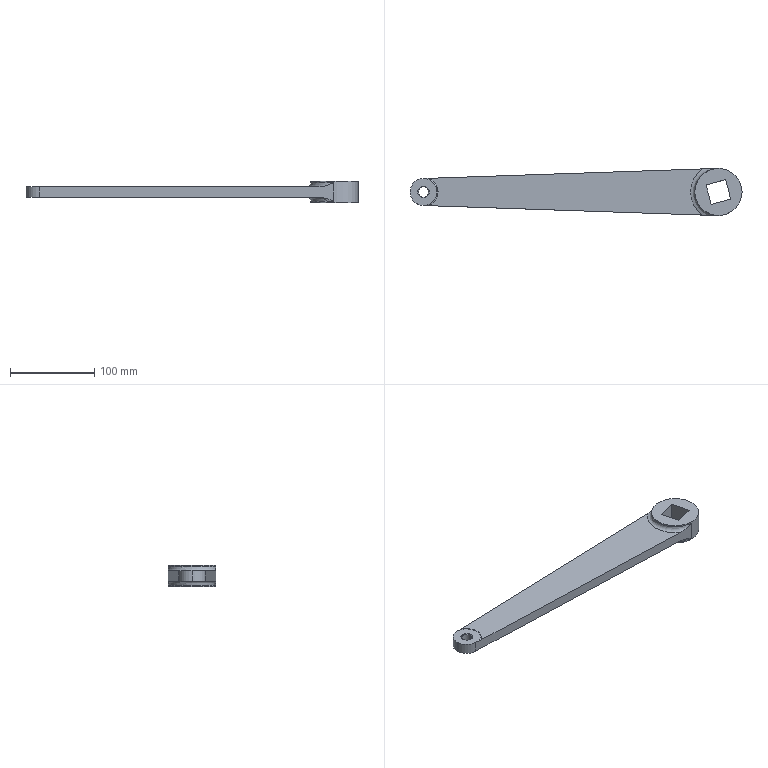Part | SolidWorks | features Boss 2, Fillet 2, Chamfer 1, Cut 1, Extrusion 1 | 1 solid | 28 faces | box 394 x 56 x 25 mm | volume 222247 mm3 | plane 12 | torus 6 | cylinder 6 | cone 4 | commonest cylinder face diameters 12 x2 32 x2 56 x2
STEP:
#1=CARTESIAN_POINT('',(-356.,0.,5.5));
#2=VERTEX_POINT('',#1);
#3=CARTESIAN_POINT('',(-344.,0.,5.5));
#4=VERTEX_POINT('',#3);
#5=CARTESIAN_POINT('',(-350.,0.,5.5));
#6=DIRECTION('',(0.,0.,1.));
#7=DIRECTION('',(1.,0.,0.));
#8=AXIS2_PLACEMENT_3D('',#5,#6,#7);
#9=CIRCLE('',#8,6.);
#10=EDGE_CURVE('',#2,#4,#9,.T.);
#11=ORIENTED_EDGE('',*,*,#10,.F.);
#12=CARTESIAN_POINT('',(-357.,0.,6.5));
#13=VERTEX_POINT('',#12);
#14=CARTESIAN_POINT('',(-356.,0.,5.5));
#15=DIRECTION('',(-0.7071,0.,0.7071));
#16=VECTOR('',#15,1000.);
#17=LINE('',#14,#16);
#18=EDGE_CURVE('',#2,#13,#17,.T.);
#19=ORIENTED_EDGE('',*,*,#18,.T.);
#20=CARTESIAN_POINT('',(-343.,0.,6.5));
#21=VERTEX_POINT('',#20);
#22=CARTESIAN_POINT('',(-350.,0.,6.5));
#23=DIRECTION('',(0.,0.,-1.));
#24=DIRECTION('',(1.,0.,0.));
#25=AXIS2_PLACEMENT_3D('',#22,#23,#24);
#26=CIRCLE('',#25,7.);
#27=EDGE_CURVE('',#21,#13,#26,.T.);
#28=ORIENTED_EDGE('',*,*,#27,.F.);
#29=CARTESIAN_POINT('',(-344.,0.,5.5));
#30=DIRECTION('',(0.7071,0.,0.7071));
#31=VECTOR('',#30,1000.);
#32=LINE('',#29,#31);
#33=EDGE_CURVE('',#4,#21,#32,.T.);
#34=ORIENTED_EDGE('',*,*,#33,.F.);
#35=EDGE_LOOP('',(#11,#19,#28,#34));
#36=FACE_OUTER_BOUND('',#35,.T.);
#37=CARTESIAN_POINT('',(-350.,0.,5.5));
#38=DIRECTION('',(0.,0.,1.));
#39=DIRECTION('',(1.,0.,0.));
#40=AXIS2_PLACEMENT_3D('',#37,#38,#39);
#41=CONICAL_SURFACE('',#40,6.,0.7854);
#42=ADVANCED_FACE('',(#36),#41,.F.);
#43=CARTESIAN_POINT('',(-344.,0.,-5.5));
#44=VERTEX_POINT('',#43);
#45=CARTESIAN_POINT('',(-356.,0.,-5.5));
#46=VERTEX_POINT('',#45);
#47=CARTESIAN_POINT('',(-350.,0.,-5.5));
#48=DIRECTION('',(0.,0.,-1.));
#49=DIRECTION('',(1.,0.,0.));
#50=AXIS2_PLACEMENT_3D('',#47,#48,#49);
#51=CIRCLE('',#50,6.);
#52=EDGE_CURVE('',#44,#46,#51,.T.);
#53=ORIENTED_EDGE('',*,*,#52,.F.);
#54=CARTESIAN_POINT('',(-343.,0.,-6.5));
#55=VERTEX_POINT('',#54);
#56=CARTESIAN_POINT('',(-343.,0.,-6.5));
#57=DIRECTION('',(0.7071,0.,-0.7071));
#58=VECTOR('',#57,1000.);
#59=LINE('',#56,#58);
#60=EDGE_CURVE('',#44,#55,#59,.T.);
#61=ORIENTED_EDGE('',*,*,#60,.T.);
#62=CARTESIAN_POINT('',(-357.,0.,-6.5));
#63=VERTEX_POINT('',#62);
#64=CARTESIAN_POINT('',(-350.,0.,-6.5));
#65=DIRECTION('',(0.,0.,1.));
#66=DIRECTION('',(1.,0.,0.));
#67=AXIS2_PLACEMENT_3D('',#64,#65,#66);
#68=CIRCLE('',#67,7.);
#69=EDGE_CURVE('',#63,#55,#68,.T.);
#70=ORIENTED_EDGE('',*,*,#69,.F.);
#71=CARTESIAN_POINT('',(-357.,0.,-6.5));
#72=DIRECTION('',(-0.7071,0.,-0.7071));
#73=VECTOR('',#72,1000.);
#74=LINE('',#71,#73);
#75=EDGE_CURVE('',#46,#63,#74,.T.);
#76=ORIENTED_EDGE('',*,*,#75,.F.);
#77=EDGE_LOOP('',(#53,#61,#70,#76));
#78=FACE_OUTER_BOUND('',#77,.T.);
#79=CARTESIAN_POINT('',(-350.,0.,-6.5));
#80=DIRECTION('',(0.,0.,-1.));
#81=DIRECTION('',(-1.,0.,0.));
#82=AXIS2_PLACEMENT_3D('',#79,#80,#81);
#83=CONICAL_SURFACE('',#82,7.,0.7854);
#84=ADVANCED_FACE('',(#78),#83,.F.);
#85=CARTESIAN_POINT('',(-332.677,0.,-6.));
#86=VERTEX_POINT('',#85);
#87=CARTESIAN_POINT('',(-343.913,16.218,-6.));
#88=VERTEX_POINT('',#87);
#89=CARTESIAN_POINT('',(-350.,0.,-6.));
#90=DIRECTION('',(0.,0.,1.));
#91=DIRECTION('',(1.,0.,0.));
#92=AXIS2_PLACEMENT_3D('',#89,#90,#91);
#93=CIRCLE('',#92,17.323);
#94=EDGE_CURVE('',#86,#88,#93,.T.);
#95=ORIENTED_EDGE('',*,*,#94,.F.);
#96=CARTESIAN_POINT('',(-334.,0.,-6.5));
#97=VERTEX_POINT('',#96);
#98=CARTESIAN_POINT('',(-332.677,0.,-8.));
#99=DIRECTION('',(0.,-1.,0.));
#100=DIRECTION('',(0.,0.,-1.));
#101=AXIS2_PLACEMENT_3D('',#98,#99,#100);
#102=CIRCLE('',#101,2.);
#103=EDGE_CURVE('',#86,#97,#102,.T.);
#104=ORIENTED_EDGE('',*,*,#103,.T.);
#105=CARTESIAN_POINT('',(-350.549,15.991,-6.5));
#106=VERTEX_POINT('',#105);
#107=CARTESIAN_POINT('',(-350.,0.,-6.5));
#108=DIRECTION('',(0.,0.,1.));
#109=DIRECTION('',(1.,0.,0.));
#110=AXIS2_PLACEMENT_3D('',#107,#108,#109);
#111=CIRCLE('',#110,16.);
#112=EDGE_CURVE('',#97,#106,#111,.T.);
#113=ORIENTED_EDGE('',*,*,#112,.T.);
#114=CARTESIAN_POINT('',(-343.913,16.218,-6.));
#115=CARTESIAN_POINT('',(-345.026,16.18,-6.));
#116=CARTESIAN_POINT('',(-346.129,16.142,-6.131));
#117=CARTESIAN_POINT('',(-347.783,16.085,-6.321));
#118=CARTESIAN_POINT('',(-348.334,16.067,-6.383));
#119=CARTESIAN_POINT('',(-349.439,16.029,-6.473));
#120=CARTESIAN_POINT('',(-349.993,16.01,-6.5));
#121=CARTESIAN_POINT('',(-350.549,15.991,-6.5));
#122=B_SPLINE_CURVE_WITH_KNOTS('',3,(#114,#115,#116,#117,#118,#119,#120,#121),.UNSPECIFIED.,.F.,.F.,(4,2,2,4),(0.,0.00333,0.004995,0.00666),.UNSPECIFIED.);
#123=EDGE_CURVE('',#88,#106,#122,.T.);
#124=ORIENTED_EDGE('',*,*,#123,.F.);
#125=EDGE_LOOP('',(#95,#104,#113,#124));
#126=FACE_OUTER_BOUND('',#125,.T.);
#127=CARTESIAN_POINT('',(-350.,0.,-8.));
#128=DIRECTION('',(0.,0.,1.));
#129=DIRECTION('',(1.,0.,0.));
#130=AXIS2_PLACEMENT_3D('',#127,#128,#129);
#131=TOROIDAL_SURFACE('',#130,17.323,2.);
#132=ADVANCED_FACE('',(#126),#131,.F.);
#133=CARTESIAN_POINT('',(-334.,0.,6.5));
#134=VERTEX_POINT('',#133);
#135=CARTESIAN_POINT('',(-350.549,15.991,6.5));
#136=VERTEX_POINT('',#135);
#137=CARTESIAN_POINT('',(-350.,0.,6.5));
#138=DIRECTION('',(0.,0.,1.));
#139=DIRECTION('',(1.,0.,0.));
#140=AXIS2_PLACEMENT_3D('',#137,#138,#139);
#141=CIRCLE('',#140,16.);
#142=EDGE_CURVE('',#134,#136,#141,.T.);
#143=ORIENTED_EDGE('',*,*,#142,.F.);
#144=CARTESIAN_POINT('',(-332.677,0.,6.));
#145=VERTEX_POINT('',#144);
#146=CARTESIAN_POINT('',(-332.677,0.,8.));
#147=DIRECTION('',(0.,-1.,0.));
#148=DIRECTION('',(0.,0.,-1.));
#149=AXIS2_PLACEMENT_3D('',#146,#147,#148);
#150=CIRCLE('',#149,2.);
#151=EDGE_CURVE('',#134,#145,#150,.T.);
#152=ORIENTED_EDGE('',*,*,#151,.T.);
#153=CARTESIAN_POINT('',(-343.913,16.218,6.));
#154=VERTEX_POINT('',#153);
#155=CARTESIAN_POINT('',(-350.,0.,6.));
#156=DIRECTION('',(0.,0.,-1.));
#157=DIRECTION('',(1.,0.,0.));
#158=AXIS2_PLACEMENT_3D('',#155,#156,#157);
#159=CIRCLE('',#158,17.323);
#160=EDGE_CURVE('',#154,#145,#159,.T.);
#161=ORIENTED_EDGE('',*,*,#160,.F.);
#162=CARTESIAN_POINT('',(-350.549,15.991,6.5));
#163=CARTESIAN_POINT('',(-349.992,16.01,6.5));
#164=CARTESIAN_POINT('',(-349.438,16.029,6.473));
#165=CARTESIAN_POINT('',(-348.332,16.067,6.383));
#166=CARTESIAN_POINT('',(-347.781,16.086,6.321));
#167=CARTESIAN_POINT('',(-346.127,16.142,6.131));
#168=CARTESIAN_POINT('',(-345.024,16.18,6.));
#169=CARTESIAN_POINT('',(-343.913,16.218,6.));
#170=B_SPLINE_CURVE_WITH_KNOTS('',3,(#162,#163,#164,#165,#166,#167,#168,#169),.UNSPECIFIED.,.F.,.F.,(4,2,2,4),(0.,0.001665,0.00333,0.006659),.UNSPECIFIED.);
#171=EDGE_CURVE('',#136,#154,#170,.T.);
#172=ORIENTED_EDGE('',*,*,#171,.F.);
#173=EDGE_LOOP('',(#143,#152,#161,#172));
#174=FACE_OUTER_BOUND('',#173,.T.);
#175=CARTESIAN_POINT('',(-350.,0.,8.));
#176=DIRECTION('',(0.,0.,1.));
#177=DIRECTION('',(1.,0.,0.));
#178=AXIS2_PLACEMENT_3D('',#175,#176,#177);
#179=TOROIDAL_SURFACE('',#178,17.323,2.);
#180=ADVANCED_FACE('',(#174),#179,.F.);
#181=ORIENTED_EDGE('',*,*,#52,.T.);
#182=CARTESIAN_POINT('',(-356.,0.,-12.5));
#183=DIRECTION('',(0.,0.,1.));
#184=VECTOR('',#183,1000.);
#185=LINE('',#182,#184);
#186=EDGE_CURVE('',#46,#2,#185,.T.);
#187=ORIENTED_EDGE('',*,*,#186,.T.);
#188=ORIENTED_EDGE('',*,*,#10,.T.);
#189=CARTESIAN_POINT('',(-344.,0.,-12.5));
#190=DIRECTION('',(0.,0.,1.));
#191=VECTOR('',#190,1000.);
#192=LINE('',#189,#191);
#193=EDGE_CURVE('',#44,#4,#192,.T.);
#194=ORIENTED_EDGE('',*,*,#193,.F.);
#195=EDGE_LOOP('',(#181,#187,#188,#194));
#196=FACE_OUTER_BOUND('',#195,.T.);
#197=CARTESIAN_POINT('',(-350.,0.,-12.5));
#198=DIRECTION('',(0.,0.,1.));
#199=DIRECTION('',(1.,0.,0.));
#200=AXIS2_PLACEMENT_3D('',#197,#198,#199);
#201=CYLINDRICAL_SURFACE('',#200,6.);
#202=ADVANCED_FACE('',(#196),#201,.F.);
#203=CARTESIAN_POINT('',(-366.,0.,6.5));
#204=VERTEX_POINT('',#203);
#205=CARTESIAN_POINT('',(-350.549,-15.991,6.5));
#206=VERTEX_POINT('',#205);
#207=CARTESIAN_POINT('',(-350.,0.,6.5));
#208=DIRECTION('',(0.,0.,1.));
#209=DIRECTION('',(1.,0.,0.));
#210=AXIS2_PLACEMENT_3D('',#207,#208,#209);
#211=CIRCLE('',#210,16.);
#212=EDGE_CURVE('',#204,#206,#211,.T.);
#213=ORIENTED_EDGE('',*,*,#212,.F.);
#214=CARTESIAN_POINT('',(-366.,0.,-6.5));
#215=VERTEX_POINT('',#214);
#216=CARTESIAN_POINT('',(-366.,0.,6.5));
#217=DIRECTION('',(0.,0.,-1.));
#218=VECTOR('',#217,1000.);
#219=LINE('',#216,#218);
#220=EDGE_CURVE('',#204,#215,#219,.T.);
#221=ORIENTED_EDGE('',*,*,#220,.T.);
#222=CARTESIAN_POINT('',(-350.549,-15.991,-6.5));
#223=VERTEX_POINT('',#222);
#224=CARTESIAN_POINT('',(-350.,0.,-6.5));
#225=DIRECTION('',(0.,0.,1.));
#226=DIRECTION('',(1.,0.,0.));
#227=AXIS2_PLACEMENT_3D('',#224,#225,#226);
#228=CIRCLE('',#227,16.);
#229=EDGE_CURVE('',#215,#223,#228,.T.);
#230=ORIENTED_EDGE('',*,*,#229,.T.);
#231=CARTESIAN_POINT('',(-350.549,-15.991,6.));
#232=DIRECTION('',(0.,0.,-1.));
#233=VECTOR('',#232,1000.);
#234=LINE('',#231,#233);
#235=EDGE_CURVE('',#206,#223,#234,.T.);
#236=ORIENTED_EDGE('',*,*,#235,.F.);
#237=EDGE_LOOP('',(#213,#221,#230,#236));
#238=FACE_OUTER_BOUND('',#237,.T.);
#239=CARTESIAN_POINT('',(-350.,0.,6.5));
#240=DIRECTION('',(0.,0.,-1.));
#241=DIRECTION('',(-1.,0.,0.));
#242=AXIS2_PLACEMENT_3D('',#239,#240,#241);
#243=CYLINDRICAL_SURFACE('',#242,16.);
#244=ADVANCED_FACE('',(#238),#243,.T.);
#245=CARTESIAN_POINT('',(28.,0.,12.5));
#246=VERTEX_POINT('',#245);
#247=CARTESIAN_POINT('',(-28.,0.,12.5));
#248=VERTEX_POINT('',#247);
#249=CARTESIAN_POINT('',(0.,0.,12.5));
#250=DIRECTION('',(0.,0.,1.));
#251=DIRECTION('',(1.,0.,0.));
#252=AXIS2_PLACEMENT_3D('',#249,#250,#251);
#253=CIRCLE('',#252,28.);
#254=EDGE_CURVE('',#246,#248,#253,.T.);
#255=ORIENTED_EDGE('',*,*,#254,.F.);
#256=CARTESIAN_POINT('',(28.,0.,-12.5));
#257=VERTEX_POINT('',#256);
#258=CARTESIAN_POINT('',(28.,0.,12.5));
#259=DIRECTION('',(0.,0.,-1.));
#260=VECTOR('',#259,1000.);
#261=LINE('',#258,#260);
#262=EDGE_CURVE('',#246,#257,#261,.T.);
#263=ORIENTED_EDGE('',*,*,#262,.T.);
#264=CARTESIAN_POINT('',(-28.,0.,-12.5));
#265=VERTEX_POINT('',#264);
#266=CARTESIAN_POINT('',(0.,0.,-12.5));
#267=DIRECTION('',(0.,0.,1.));
#268=DIRECTION('',(1.,0.,0.));
#269=AXIS2_PLACEMENT_3D('',#266,#267,#268);
#270=CIRCLE('',#269,28.);
#271=EDGE_CURVE('',#257,#265,#270,.T.);
#272=ORIENTED_EDGE('',*,*,#271,.T.);
#273=CARTESIAN_POINT('',(-28.,0.,-11.));
#274=VERTEX_POINT('',#273);
#275=CARTESIAN_POINT('',(-28.,0.,12.5));
#276=DIRECTION('',(0.,0.,-1.));
#277=VECTOR('',#276,1000.);
#278=LINE('',#275,#277);
#279=EDGE_CURVE('',#274,#265,#278,.T.);
#280=ORIENTED_EDGE('',*,*,#279,.F.);
#281=CARTESIAN_POINT('',(-0.96,27.984,-11.));
#282=VERTEX_POINT('',#281);
#283=CARTESIAN_POINT('',(0.,0.,-11.));
#284=DIRECTION('',(0.,0.,-1.));
#285=DIRECTION('',(1.,0.,0.));
#286=AXIS2_PLACEMENT_3D('',#283,#284,#285);
#287=CIRCLE('',#286,28.);
#288=EDGE_CURVE('',#274,#282,#287,.T.);
#289=ORIENTED_EDGE('',*,*,#288,.T.);
#290=CARTESIAN_POINT('',(-0.96,27.984,11.));
#291=VERTEX_POINT('',#290);
#292=CARTESIAN_POINT('',(-0.96,27.984,6.));
#293=DIRECTION('',(0.,0.,-1.));
#294=VECTOR('',#293,1000.);
#295=LINE('',#292,#294);
#296=EDGE_CURVE('',#291,#282,#295,.T.);
#297=ORIENTED_EDGE('',*,*,#296,.F.);
#298=CARTESIAN_POINT('',(-28.,0.,11.));
#299=VERTEX_POINT('',#298);
#300=CARTESIAN_POINT('',(0.,0.,11.));
#301=DIRECTION('',(0.,0.,1.));
#302=DIRECTION('',(1.,0.,0.));
#303=AXIS2_PLACEMENT_3D('',#300,#301,#302);
#304=CIRCLE('',#303,28.);
#305=EDGE_CURVE('',#291,#299,#304,.T.);
#306=ORIENTED_EDGE('',*,*,#305,.T.);
#307=CARTESIAN_POINT('',(-28.,0.,12.5));
#308=DIRECTION('',(0.,0.,-1.));
#309=VECTOR('',#308,1000.);
#310=LINE('',#307,#309);
#311=EDGE_CURVE('',#248,#299,#310,.T.);
#312=ORIENTED_EDGE('',*,*,#311,.F.);
#313=EDGE_LOOP('',(#255,#263,#272,#280,#289,#297,#306,#312));
#314=FACE_OUTER_BOUND('',#313,.T.);
#315=CARTESIAN_POINT('',(0.,0.,12.5));
#316=DIRECTION('',(0.,0.,-1.));
#317=DIRECTION('',(-1.,0.,0.));
#318=AXIS2_PLACEMENT_3D('',#315,#316,#317);
#319=CYLINDRICAL_SURFACE('',#318,28.);
#320=ADVANCED_FACE('',(#314),#319,.T.);
#321=CARTESIAN_POINT('',(-18.414,-27.385,-6.));
#322=VERTEX_POINT('',#321);
#323=CARTESIAN_POINT('',(-343.913,-16.218,-6.));
#324=VERTEX_POINT('',#323);
#325=CARTESIAN_POINT('',(-159.15,-22.557,-6.));
#326=DIRECTION('',(-0.9994,0.03429,0.));
#327=VECTOR('',#326,1000.);
#328=LINE('',#325,#327);
#329=EDGE_CURVE('',#322,#324,#328,.T.);
#330=ORIENTED_EDGE('',*,*,#329,.F.);
#331=CARTESIAN_POINT('',(-0.96,-27.984,-11.));
#332=VERTEX_POINT('',#331);
#333=CARTESIAN_POINT('',(-18.414,-27.385,-6.));
#334=CARTESIAN_POINT('',(-17.645,-27.411,-6.));
#335=CARTESIAN_POINT('',(-16.885,-27.437,-6.049));
#336=CARTESIAN_POINT('',(-15.376,-27.489,-6.219));
#337=CARTESIAN_POINT('',(-14.628,-27.515,-6.34));
#338=CARTESIAN_POINT('',(-13.141,-27.566,-6.639));
#339=CARTESIAN_POINT('',(-12.402,-27.591,-6.816));
#340=CARTESIAN_POINT('',(-10.932,-27.641,-7.215));
#341=CARTESIAN_POINT('',(-10.2,-27.667,-7.436));
#342=CARTESIAN_POINT('',(-8.025,-27.741,-8.147));
#343=CARTESIAN_POINT('',(-6.599,-27.79,-8.683));
#344=CARTESIAN_POINT('',(-4.476,-27.863,-9.53));
#345=CARTESIAN_POINT('',(-3.771,-27.887,-9.82));
#346=CARTESIAN_POINT('',(-2.716,-27.923,-10.26));
#347=CARTESIAN_POINT('',(-2.364,-27.935,-10.407));
#348=CARTESIAN_POINT('',(-1.662,-27.959,-10.703));
#349=CARTESIAN_POINT('',(-1.309,-27.972,-10.852));
#350=CARTESIAN_POINT('',(-0.96,-27.984,-11.));
#351=B_SPLINE_CURVE_WITH_KNOTS('',3,(#333,#334,#335,#336,#337,#338,#339,#340,#341,#342,#343,#344,#345,#346,#347,#348,#349,#350),.UNSPECIFIED.,.F.,.F.,(4,2,2,2,2,2,2,2,4),(0.,0.002275,0.00455,0.006826,0.009101,0.01365,0.01593,0.01706,0.0182),.UNSPECIFIED.);
#352=EDGE_CURVE('',#322,#332,#351,.T.);
#353=ORIENTED_EDGE('',*,*,#352,.T.);
#354=CARTESIAN_POINT('',(-0.96,-27.984,11.));
#355=VERTEX_POINT('',#354);
#356=CARTESIAN_POINT('',(-0.96,-27.984,6.));
#357=DIRECTION('',(0.,0.,-1.));
#358=VECTOR('',#357,1000.);
#359=LINE('',#356,#358);
#360=EDGE_CURVE('',#355,#332,#359,.T.);
#361=ORIENTED_EDGE('',*,*,#360,.F.);
#362=CARTESIAN_POINT('',(-18.414,-27.385,6.));
#363=VERTEX_POINT('',#362);
#364=CARTESIAN_POINT('',(-0.96,-27.984,11.));
#365=CARTESIAN_POINT('',(-2.363,-27.935,10.407));
#366=CARTESIAN_POINT('',(-3.768,-27.887,9.812));
#367=CARTESIAN_POINT('',(-6.599,-27.79,8.683));
#368=CARTESIAN_POINT('',(-8.025,-27.741,8.147));
#369=CARTESIAN_POINT('',(-10.2,-27.667,7.436));
#370=CARTESIAN_POINT('',(-10.932,-27.641,7.215));
#371=CARTESIAN_POINT('',(-12.402,-27.591,6.816));
#372=CARTESIAN_POINT('',(-13.141,-27.566,6.639));
#373=CARTESIAN_POINT('',(-14.628,-27.515,6.34));
#374=CARTESIAN_POINT('',(-15.376,-27.489,6.219));
#375=CARTESIAN_POINT('',(-16.885,-27.437,6.049));
#376=CARTESIAN_POINT('',(-17.645,-27.411,6.));
#377=CARTESIAN_POINT('',(-18.414,-27.385,6.));
#378=B_SPLINE_CURVE_WITH_KNOTS('',3,(#364,#365,#366,#367,#368,#369,#370,#371,#372,#373,#374,#375,#376,#377),.UNSPECIFIED.,.F.,.F.,(4,2,2,2,2,2,4),(-0.00003347,0.00454,0.009113,0.0114,0.01369,0.01597,0.01826),.UNSPECIFIED.);
#379=EDGE_CURVE('',#355,#363,#378,.T.);
#380=ORIENTED_EDGE('',*,*,#379,.T.);
#381=CARTESIAN_POINT('',(-343.913,-16.218,6.));
#382=VERTEX_POINT('',#381);
#383=CARTESIAN_POINT('',(-159.15,-22.557,6.));
#384=DIRECTION('',(-0.9994,0.03429,0.));
#385=VECTOR('',#384,1000.);
#386=LINE('',#383,#385);
#387=EDGE_CURVE('',#363,#382,#386,.T.);
#388=ORIENTED_EDGE('',*,*,#387,.T.);
#389=CARTESIAN_POINT('',(-343.913,-16.218,6.));
#390=CARTESIAN_POINT('',(-345.026,-16.18,6.));
#391=CARTESIAN_POINT('',(-346.129,-16.142,6.131));
#392=CARTESIAN_POINT('',(-347.783,-16.085,6.321));
#393=CARTESIAN_POINT('',(-348.334,-16.067,6.383));
#394=CARTESIAN_POINT('',(-349.439,-16.029,6.473));
#395=CARTESIAN_POINT('',(-349.993,-16.01,6.5));
#396=CARTESIAN_POINT('',(-350.549,-15.991,6.5));
#397=B_SPLINE_CURVE_WITH_KNOTS('',3,(#389,#390,#391,#392,#393,#394,#395,#396),.UNSPECIFIED.,.F.,.F.,(4,2,2,4),(0.,0.00333,0.004995,0.00666),.UNSPECIFIED.);
#398=EDGE_CURVE('',#382,#206,#397,.T.);
#399=ORIENTED_EDGE('',*,*,#398,.T.);
#400=ORIENTED_EDGE('',*,*,#235,.T.);
#401=CARTESIAN_POINT('',(-350.549,-15.991,-6.5));
#402=CARTESIAN_POINT('',(-349.992,-16.01,-6.5));
#403=CARTESIAN_POINT('',(-349.438,-16.029,-6.473));
#404=CARTESIAN_POINT('',(-348.332,-16.067,-6.383));
#405=CARTESIAN_POINT('',(-347.781,-16.086,-6.321));
#406=CARTESIAN_POINT('',(-346.127,-16.142,-6.131));
#407=CARTESIAN_POINT('',(-345.024,-16.18,-6.));
#408=CARTESIAN_POINT('',(-343.913,-16.218,-6.));
#409=B_SPLINE_CURVE_WITH_KNOTS('',3,(#401,#402,#403,#404,#405,#406,#407,#408),.UNSPECIFIED.,.F.,.F.,(4,2,2,4),(0.,0.001665,0.00333,0.006659),.UNSPECIFIED.);
#410=EDGE_CURVE('',#223,#324,#409,.T.);
#411=ORIENTED_EDGE('',*,*,#410,.T.);
#412=EDGE_LOOP('',(#330,#353,#361,#380,#388,#399,#400,#411));
#413=FACE_OUTER_BOUND('',#412,.T.);
#414=CARTESIAN_POINT('',(-159.15,-22.557,6.));
#415=DIRECTION('',(-0.03429,-0.9994,0.));
#416=DIRECTION('',(0.9994,-0.03429,0.));
#417=AXIS2_PLACEMENT_3D('',#414,#415,#416);
#418=PLANE('',#417);
#419=ADVANCED_FACE('',(#413),#418,.T.);
#420=ORIENTED_EDGE('',*,*,#296,.T.);
#421=CARTESIAN_POINT('',(-18.414,27.385,-6.));
#422=VERTEX_POINT('',#421);
#423=CARTESIAN_POINT('',(-0.96,27.984,-11.));
#424=CARTESIAN_POINT('',(-2.363,27.935,-10.407));
#425=CARTESIAN_POINT('',(-3.768,27.887,-9.812));
#426=CARTESIAN_POINT('',(-6.599,27.79,-8.683));
#427=CARTESIAN_POINT('',(-8.025,27.741,-8.147));
#428=CARTESIAN_POINT('',(-10.2,27.667,-7.436));
#429=CARTESIAN_POINT('',(-10.932,27.641,-7.215));
#430=CARTESIAN_POINT('',(-12.402,27.591,-6.816));
#431=CARTESIAN_POINT('',(-13.141,27.566,-6.639));
#432=CARTESIAN_POINT('',(-14.628,27.515,-6.34));
#433=CARTESIAN_POINT('',(-15.376,27.489,-6.219));
#434=CARTESIAN_POINT('',(-16.885,27.437,-6.049));
#435=CARTESIAN_POINT('',(-17.645,27.411,-6.));
#436=CARTESIAN_POINT('',(-18.414,27.385,-6.));
#437=B_SPLINE_CURVE_WITH_KNOTS('',3,(#423,#424,#425,#426,#427,#428,#429,#430,#431,#432,#433,#434,#435,#436),.UNSPECIFIED.,.F.,.F.,(4,2,2,2,2,2,4),(-0.00003347,0.00454,0.009113,0.0114,0.01369,0.01597,0.01826),.UNSPECIFIED.);
#438=EDGE_CURVE('',#282,#422,#437,.T.);
#439=ORIENTED_EDGE('',*,*,#438,.T.);
#440=CARTESIAN_POINT('',(-180.373,21.829,-6.));
#441=DIRECTION('',(-0.9994,-0.03429,0.));
#442=VECTOR('',#441,1000.);
#443=LINE('',#440,#442);
#444=EDGE_CURVE('',#422,#88,#443,.T.);
#445=ORIENTED_EDGE('',*,*,#444,.T.);
#446=ORIENTED_EDGE('',*,*,#123,.T.);
#447=CARTESIAN_POINT('',(-350.549,15.991,6.));
#448=DIRECTION('',(0.,0.,-1.));
#449=VECTOR('',#448,1000.);
#450=LINE('',#447,#449);
#451=EDGE_CURVE('',#136,#106,#450,.T.);
#452=ORIENTED_EDGE('',*,*,#451,.F.);
#453=ORIENTED_EDGE('',*,*,#171,.T.);
#454=CARTESIAN_POINT('',(-18.414,27.385,6.));
#455=VERTEX_POINT('',#454);
#456=CARTESIAN_POINT('',(-180.373,21.829,6.));
#457=DIRECTION('',(-0.9994,-0.03429,0.));
#458=VECTOR('',#457,1000.);
#459=LINE('',#456,#458);
#460=EDGE_CURVE('',#455,#154,#459,.T.);
#461=ORIENTED_EDGE('',*,*,#460,.F.);
#462=CARTESIAN_POINT('',(-18.414,27.385,6.));
#463=CARTESIAN_POINT('',(-17.645,27.411,6.));
#464=CARTESIAN_POINT('',(-16.885,27.437,6.049));
#465=CARTESIAN_POINT('',(-15.376,27.489,6.219));
#466=CARTESIAN_POINT('',(-14.628,27.515,6.34));
#467=CARTESIAN_POINT('',(-13.141,27.566,6.639));
#468=CARTESIAN_POINT('',(-12.402,27.591,6.816));
#469=CARTESIAN_POINT('',(-10.932,27.641,7.215));
#470=CARTESIAN_POINT('',(-10.2,27.667,7.436));
#471=CARTESIAN_POINT('',(-8.025,27.741,8.147));
#472=CARTESIAN_POINT('',(-6.599,27.79,8.683));
#473=CARTESIAN_POINT('',(-4.476,27.863,9.53));
#474=CARTESIAN_POINT('',(-3.771,27.887,9.82));
#475=CARTESIAN_POINT('',(-2.716,27.923,10.26));
#476=CARTESIAN_POINT('',(-2.364,27.935,10.407));
#477=CARTESIAN_POINT('',(-1.662,27.959,10.703));
#478=CARTESIAN_POINT('',(-1.309,27.972,10.852));
#479=CARTESIAN_POINT('',(-0.96,27.984,11.));
#480=B_SPLINE_CURVE_WITH_KNOTS('',3,(#462,#463,#464,#465,#466,#467,#468,#469,#470,#471,#472,#473,#474,#475,#476,#477,#478,#479),.UNSPECIFIED.,.F.,.F.,(4,2,2,2,2,2,2,2,4),(0.,0.002275,0.00455,0.006826,0.009101,0.01365,0.01593,0.01706,0.0182),.UNSPECIFIED.);
#481=EDGE_CURVE('',#455,#291,#480,.T.);
#482=ORIENTED_EDGE('',*,*,#481,.T.);
#483=EDGE_LOOP('',(#420,#439,#445,#446,#452,#453,#461,#482));
#484=FACE_OUTER_BOUND('',#483,.T.);
#485=CARTESIAN_POINT('',(-180.373,21.829,6.));
#486=DIRECTION('',(0.03429,-0.9994,0.));
#487=DIRECTION('',(0.9994,0.03429,0.));
#488=AXIS2_PLACEMENT_3D('',#485,#486,#487);
#489=PLANE('',#488);
#490=ADVANCED_FACE('',(#484),#489,.F.);
#491=ORIENTED_EDGE('',*,*,#460,.T.);
#492=ORIENTED_EDGE('',*,*,#160,.T.);
#493=CARTESIAN_POINT('',(-350.,0.,6.));
#494=DIRECTION('',(0.,0.,-1.));
#495=DIRECTION('',(1.,0.,0.));
#496=AXIS2_PLACEMENT_3D('',#493,#494,#495);
#497=CIRCLE('',#496,17.323);
#498=EDGE_CURVE('',#145,#382,#497,.T.);
#499=ORIENTED_EDGE('',*,*,#498,.T.);
#500=ORIENTED_EDGE('',*,*,#387,.F.);
#501=CARTESIAN_POINT('',(0.,0.,6.));
#502=DIRECTION('',(0.,0.,-1.));
#503=DIRECTION('',(1.,0.,0.));
#504=AXIS2_PLACEMENT_3D('',#501,#502,#503);
#505=CIRCLE('',#504,33.);
#506=EDGE_CURVE('',#363,#455,#505,.T.);
#507=ORIENTED_EDGE('',*,*,#506,.T.);
#508=EDGE_LOOP('',(#491,#492,#499,#500,#507));
#509=FACE_OUTER_BOUND('',#508,.T.);
#510=CARTESIAN_POINT('',(-169.,-309.681,6.));
#511=DIRECTION('',(0.,0.,1.));
#512=DIRECTION('',(1.,0.,0.));
#513=AXIS2_PLACEMENT_3D('',#510,#511,#512);
#514=PLANE('',#513);
#515=ADVANCED_FACE('',(#509),#514,.T.);
#516=ORIENTED_EDGE('',*,*,#329,.T.);
#517=CARTESIAN_POINT('',(-350.,0.,-6.));
#518=DIRECTION('',(0.,0.,1.));
#519=DIRECTION('',(1.,0.,0.));
#520=AXIS2_PLACEMENT_3D('',#517,#518,#519);
#521=CIRCLE('',#520,17.323);
#522=EDGE_CURVE('',#324,#86,#521,.T.);
#523=ORIENTED_EDGE('',*,*,#522,.T.);
#524=ORIENTED_EDGE('',*,*,#94,.T.);
#525=ORIENTED_EDGE('',*,*,#444,.F.);
#526=CARTESIAN_POINT('',(0.,0.,-6.));
#527=DIRECTION('',(0.,0.,1.));
#528=DIRECTION('',(1.,0.,0.));
#529=AXIS2_PLACEMENT_3D('',#526,#527,#528);
#530=CIRCLE('',#529,33.);
#531=EDGE_CURVE('',#422,#322,#530,.T.);
#532=ORIENTED_EDGE('',*,*,#531,.T.);
#533=EDGE_LOOP('',(#516,#523,#524,#525,#532));
#534=FACE_OUTER_BOUND('',#533,.T.);
#535=CARTESIAN_POINT('',(-169.,-309.681,-6.));
#536=DIRECTION('',(0.,0.,1.));
#537=DIRECTION('',(1.,0.,0.));
#538=AXIS2_PLACEMENT_3D('',#535,#536,#537);
#539=PLANE('',#538);
#540=ADVANCED_FACE('',(#534),#539,.F.);
#541=ORIENTED_EDGE('',*,*,#262,.F.);
#542=CARTESIAN_POINT('',(0.,0.,12.5));
#543=DIRECTION('',(0.,0.,1.));
#544=DIRECTION('',(1.,0.,0.));
#545=AXIS2_PLACEMENT_3D('',#542,#543,#544);
#546=CIRCLE('',#545,28.);
#547=EDGE_CURVE('',#248,#246,#546,.T.);
#548=ORIENTED_EDGE('',*,*,#547,.F.);
#549=ORIENTED_EDGE('',*,*,#311,.T.);
#550=CARTESIAN_POINT('',(0.,0.,11.));
#551=DIRECTION('',(0.,0.,1.));
#552=DIRECTION('',(1.,0.,0.));
#553=AXIS2_PLACEMENT_3D('',#550,#551,#552);
#554=CIRCLE('',#553,28.);
#555=EDGE_CURVE('',#299,#355,#554,.T.);
#556=ORIENTED_EDGE('',*,*,#555,.T.);
#557=ORIENTED_EDGE('',*,*,#360,.T.);
#558=CARTESIAN_POINT('',(0.,0.,-11.));
#559=DIRECTION('',(0.,0.,-1.));
#560=DIRECTION('',(1.,0.,0.));
#561=AXIS2_PLACEMENT_3D('',#558,#559,#560);
#562=CIRCLE('',#561,28.);
#563=EDGE_CURVE('',#332,#274,#562,.T.);
#564=ORIENTED_EDGE('',*,*,#563,.T.);
#565=ORIENTED_EDGE('',*,*,#279,.T.);
#566=CARTESIAN_POINT('',(0.,0.,-12.5));
#567=DIRECTION('',(0.,0.,1.));
#568=DIRECTION('',(1.,0.,0.));
#569=AXIS2_PLACEMENT_3D('',#566,#567,#568);
#570=CIRCLE('',#569,28.);
#571=EDGE_CURVE('',#265,#257,#570,.T.);
#572=ORIENTED_EDGE('',*,*,#571,.T.);
#573=EDGE_LOOP('',(#541,#548,#549,#556,#557,#564,#565,#572));
#574=FACE_OUTER_BOUND('',#573,.T.);
#575=CARTESIAN_POINT('',(0.,0.,12.5));
#576=DIRECTION('',(0.,0.,-1.));
#577=DIRECTION('',(-1.,0.,0.));
#578=AXIS2_PLACEMENT_3D('',#575,#576,#577);
#579=CYLINDRICAL_SURFACE('',#578,28.);
#580=ADVANCED_FACE('',(#574),#579,.T.);
#581=CARTESIAN_POINT('',(-14.697,8.485,12.5));
#582=VERTEX_POINT('',#581);
#583=CARTESIAN_POINT('',(-8.485,-14.697,12.5));
#584=VERTEX_POINT('',#583);
#585=CARTESIAN_POINT('',(-14.697,8.485,12.5));
#586=DIRECTION('',(0.2588,-0.9659,0.));
#587=VECTOR('',#586,1000.);
#588=LINE('',#585,#587);
#589=EDGE_CURVE('',#582,#584,#588,.T.);
#590=ORIENTED_EDGE('',*,*,#589,.F.);
#591=CARTESIAN_POINT('',(8.485,14.697,12.5));
#592=VERTEX_POINT('',#591);
#593=CARTESIAN_POINT('',(-14.697,8.485,12.5));
#594=DIRECTION('',(-0.9659,-0.2588,0.));
#595=VECTOR('',#594,1000.);
#596=LINE('',#593,#595);
#597=EDGE_CURVE('',#592,#582,#596,.T.);
#598=ORIENTED_EDGE('',*,*,#597,.F.);
#599=CARTESIAN_POINT('',(14.697,-8.485,12.5));
#600=VERTEX_POINT('',#599);
#601=CARTESIAN_POINT('',(8.485,14.697,12.5));
#602=DIRECTION('',(-0.2588,0.9659,0.));
#603=VECTOR('',#602,1000.);
#604=LINE('',#601,#603);
#605=EDGE_CURVE('',#600,#592,#604,.T.);
#606=ORIENTED_EDGE('',*,*,#605,.F.);
#607=CARTESIAN_POINT('',(-8.485,-14.697,12.5));
#608=DIRECTION('',(0.9659,0.2588,0.));
#609=VECTOR('',#608,1000.);
#610=LINE('',#607,#609);
#611=EDGE_CURVE('',#584,#600,#610,.T.);
#612=ORIENTED_EDGE('',*,*,#611,.F.);
#613=EDGE_LOOP('',(#590,#598,#606,#612));
#614=FACE_BOUND('',#613,.T.);
#615=ORIENTED_EDGE('',*,*,#547,.T.);
#616=ORIENTED_EDGE('',*,*,#254,.T.);
#617=EDGE_LOOP('',(#615,#616));
#618=FACE_OUTER_BOUND('',#617,.T.);
#619=CARTESIAN_POINT('',(-169.,-309.681,12.5));
#620=DIRECTION('',(0.,0.,1.));
#621=DIRECTION('',(1.,0.,0.));
#622=AXIS2_PLACEMENT_3D('',#619,#620,#621);
#623=PLANE('',#622);
#624=ADVANCED_FACE('',(#614,#618),#623,.T.);
#625=CARTESIAN_POINT('',(8.485,14.697,-12.5));
#626=VERTEX_POINT('',#625);
#627=CARTESIAN_POINT('',(-14.697,8.485,-12.5));
#628=VERTEX_POINT('',#627);
#629=CARTESIAN_POINT('',(-14.697,8.485,-12.5));
#630=DIRECTION('',(-0.9659,-0.2588,0.));
#631=VECTOR('',#630,1000.);
#632=LINE('',#629,#631);
#633=EDGE_CURVE('',#626,#628,#632,.T.);
#634=ORIENTED_EDGE('',*,*,#633,.T.);
#635=CARTESIAN_POINT('',(-8.485,-14.697,-12.5));
#636=VERTEX_POINT('',#635);
#637=CARTESIAN_POINT('',(-14.697,8.485,-12.5));
#638=DIRECTION('',(0.2588,-0.9659,0.));
#639=VECTOR('',#638,1000.);
#640=LINE('',#637,#639);
#641=EDGE_CURVE('',#628,#636,#640,.T.);
#642=ORIENTED_EDGE('',*,*,#641,.T.);
#643=CARTESIAN_POINT('',(14.697,-8.485,-12.5));
#644=VERTEX_POINT('',#643);
#645=CARTESIAN_POINT('',(-8.485,-14.697,-12.5));
#646=DIRECTION('',(0.9659,0.2588,0.));
#647=VECTOR('',#646,1000.);
#648=LINE('',#645,#647);
#649=EDGE_CURVE('',#636,#644,#648,.T.);
#650=ORIENTED_EDGE('',*,*,#649,.T.);
#651=CARTESIAN_POINT('',(8.485,14.697,-12.5));
#652=DIRECTION('',(-0.2588,0.9659,0.));
#653=VECTOR('',#652,1000.);
#654=LINE('',#651,#653);
#655=EDGE_CURVE('',#644,#626,#654,.T.);
#656=ORIENTED_EDGE('',*,*,#655,.T.);
#657=EDGE_LOOP('',(#634,#642,#650,#656));
#658=FACE_BOUND('',#657,.T.);
#659=ORIENTED_EDGE('',*,*,#571,.F.);
#660=ORIENTED_EDGE('',*,*,#271,.F.);
#661=EDGE_LOOP('',(#659,#660));
#662=FACE_OUTER_BOUND('',#661,.T.);
#663=CARTESIAN_POINT('',(-169.,-309.681,-12.5));
#664=DIRECTION('',(0.,0.,1.));
#665=DIRECTION('',(1.,0.,0.));
#666=AXIS2_PLACEMENT_3D('',#663,#664,#665);
#667=PLANE('',#666);
#668=ADVANCED_FACE('',(#658,#662),#667,.F.);
#669=ORIENTED_EDGE('',*,*,#220,.F.);
#670=CARTESIAN_POINT('',(-350.,0.,6.5));
#671=DIRECTION('',(0.,0.,1.));
#672=DIRECTION('',(1.,0.,0.));
#673=AXIS2_PLACEMENT_3D('',#670,#671,#672);
#674=CIRCLE('',#673,16.);
#675=EDGE_CURVE('',#136,#204,#674,.T.);
#676=ORIENTED_EDGE('',*,*,#675,.F.);
#677=ORIENTED_EDGE('',*,*,#451,.T.);
#678=CARTESIAN_POINT('',(-350.,0.,-6.5));
#679=DIRECTION('',(0.,0.,1.));
#680=DIRECTION('',(1.,0.,0.));
#681=AXIS2_PLACEMENT_3D('',#678,#679,#680);
#682=CIRCLE('',#681,16.);
#683=EDGE_CURVE('',#106,#215,#682,.T.);
#684=ORIENTED_EDGE('',*,*,#683,.T.);
#685=EDGE_LOOP('',(#669,#676,#677,#684));
#686=FACE_OUTER_BOUND('',#685,.T.);
#687=CARTESIAN_POINT('',(-350.,0.,6.5));
#688=DIRECTION('',(0.,0.,-1.));
#689=DIRECTION('',(-1.,0.,0.));
#690=AXIS2_PLACEMENT_3D('',#687,#688,#689);
#691=CYLINDRICAL_SURFACE('',#690,16.);
#692=ADVANCED_FACE('',(#686),#691,.T.);
#693=ORIENTED_EDGE('',*,*,#27,.T.);
#694=CARTESIAN_POINT('',(-350.,0.,6.5));
#695=DIRECTION('',(0.,0.,-1.));
#696=DIRECTION('',(1.,0.,0.));
#697=AXIS2_PLACEMENT_3D('',#694,#695,#696);
#698=CIRCLE('',#697,7.);
#699=EDGE_CURVE('',#13,#21,#698,.T.);
#700=ORIENTED_EDGE('',*,*,#699,.T.);
#701=EDGE_LOOP('',(#693,#700));
#702=FACE_BOUND('',#701,.T.);
#703=ORIENTED_EDGE('',*,*,#675,.T.);
#704=ORIENTED_EDGE('',*,*,#212,.T.);
#705=CARTESIAN_POINT('',(-350.,0.,6.5));
#706=DIRECTION('',(0.,0.,1.));
#707=DIRECTION('',(1.,0.,0.));
#708=AXIS2_PLACEMENT_3D('',#705,#706,#707);
#709=CIRCLE('',#708,16.);
#710=EDGE_CURVE('',#206,#134,#709,.T.);
#711=ORIENTED_EDGE('',*,*,#710,.T.);
#712=ORIENTED_EDGE('',*,*,#142,.T.);
#713=EDGE_LOOP('',(#703,#704,#711,#712));
#714=FACE_OUTER_BOUND('',#713,.T.);
#715=CARTESIAN_POINT('',(-169.,-309.681,6.5));
#716=DIRECTION('',(0.,0.,1.));
#717=DIRECTION('',(1.,0.,0.));
#718=AXIS2_PLACEMENT_3D('',#715,#716,#717);
#719=PLANE('',#718);
#720=ADVANCED_FACE('',(#702,#714),#719,.T.);
#721=ORIENTED_EDGE('',*,*,#69,.T.);
#722=CARTESIAN_POINT('',(-350.,0.,-6.5));
#723=DIRECTION('',(0.,0.,1.));
#724=DIRECTION('',(1.,0.,0.));
#725=AXIS2_PLACEMENT_3D('',#722,#723,#724);
#726=CIRCLE('',#725,7.);
#727=EDGE_CURVE('',#55,#63,#726,.T.);
#728=ORIENTED_EDGE('',*,*,#727,.T.);
#729=EDGE_LOOP('',(#721,#728));
#730=FACE_BOUND('',#729,.T.);
#731=ORIENTED_EDGE('',*,*,#683,.F.);
#732=ORIENTED_EDGE('',*,*,#112,.F.);
#733=CARTESIAN_POINT('',(-350.,0.,-6.5));
#734=DIRECTION('',(0.,0.,1.));
#735=DIRECTION('',(1.,0.,0.));
#736=AXIS2_PLACEMENT_3D('',#733,#734,#735);
#737=CIRCLE('',#736,16.);
#738=EDGE_CURVE('',#223,#97,#737,.T.);
#739=ORIENTED_EDGE('',*,*,#738,.F.);
#740=ORIENTED_EDGE('',*,*,#229,.F.);
#741=EDGE_LOOP('',(#731,#732,#739,#740));
#742=FACE_OUTER_BOUND('',#741,.T.);
#743=CARTESIAN_POINT('',(-169.,-309.681,-6.5));
#744=DIRECTION('',(0.,0.,1.));
#745=DIRECTION('',(1.,0.,0.));
#746=AXIS2_PLACEMENT_3D('',#743,#744,#745);
#747=PLANE('',#746);
#748=ADVANCED_FACE('',(#730,#742),#747,.F.);
#749=ORIENTED_EDGE('',*,*,#589,.T.);
#750=CARTESIAN_POINT('',(-8.485,-14.697,-12.5));
#751=DIRECTION('',(0.,0.,1.));
#752=VECTOR('',#751,1000.);
#753=LINE('',#750,#752);
#754=EDGE_CURVE('',#636,#584,#753,.T.);
#755=ORIENTED_EDGE('',*,*,#754,.F.);
#756=ORIENTED_EDGE('',*,*,#641,.F.);
#757=CARTESIAN_POINT('',(-14.697,8.485,-12.5));
#758=DIRECTION('',(0.,0.,1.));
#759=VECTOR('',#758,1000.);
#760=LINE('',#757,#759);
#761=EDGE_CURVE('',#628,#582,#760,.T.);
#762=ORIENTED_EDGE('',*,*,#761,.T.);
#763=EDGE_LOOP('',(#749,#755,#756,#762));
#764=FACE_OUTER_BOUND('',#763,.T.);
#765=CARTESIAN_POINT('',(-14.697,8.485,-12.5));
#766=DIRECTION('',(-0.9659,-0.2588,0.));
#767=DIRECTION('',(0.2588,-0.9659,0.));
#768=AXIS2_PLACEMENT_3D('',#765,#766,#767);
#769=PLANE('',#768);
#770=ADVANCED_FACE('',(#764),#769,.F.);
#771=ORIENTED_EDGE('',*,*,#597,.T.);
#772=ORIENTED_EDGE('',*,*,#761,.F.);
#773=ORIENTED_EDGE('',*,*,#633,.F.);
#774=CARTESIAN_POINT('',(8.485,14.697,-12.5));
#775=DIRECTION('',(0.,0.,1.));
#776=VECTOR('',#775,1000.);
#777=LINE('',#774,#776);
#778=EDGE_CURVE('',#626,#592,#777,.T.);
#779=ORIENTED_EDGE('',*,*,#778,.T.);
#780=EDGE_LOOP('',(#771,#772,#773,#779));
#781=FACE_OUTER_BOUND('',#780,.T.);
#782=CARTESIAN_POINT('',(-14.697,8.485,-12.5));
#783=DIRECTION('',(-0.2588,0.9659,0.));
#784=DIRECTION('',(-0.9659,-0.2588,0.));
#785=AXIS2_PLACEMENT_3D('',#782,#783,#784);
#786=PLANE('',#785);
#787=ADVANCED_FACE('',(#781),#786,.F.);
#788=ORIENTED_EDGE('',*,*,#605,.T.);
#789=ORIENTED_EDGE('',*,*,#778,.F.);
#790=ORIENTED_EDGE('',*,*,#655,.F.);
#791=CARTESIAN_POINT('',(14.697,-8.485,-12.5));
#792=DIRECTION('',(0.,0.,1.));
#793=VECTOR('',#792,1000.);
#794=LINE('',#791,#793);
#795=EDGE_CURVE('',#644,#600,#794,.T.);
#796=ORIENTED_EDGE('',*,*,#795,.T.);
#797=EDGE_LOOP('',(#788,#789,#790,#796));
#798=FACE_OUTER_BOUND('',#797,.T.);
#799=CARTESIAN_POINT('',(8.485,14.697,-12.5));
#800=DIRECTION('',(0.9659,0.2588,0.));
#801=DIRECTION('',(-0.2588,0.9659,0.));
#802=AXIS2_PLACEMENT_3D('',#799,#800,#801);
#803=PLANE('',#802);
#804=ADVANCED_FACE('',(#798),#803,.F.);
#805=ORIENTED_EDGE('',*,*,#611,.T.);
#806=ORIENTED_EDGE('',*,*,#795,.F.);
#807=ORIENTED_EDGE('',*,*,#649,.F.);
#808=ORIENTED_EDGE('',*,*,#754,.T.);
#809=EDGE_LOOP('',(#805,#806,#807,#808));
#810=FACE_OUTER_BOUND('',#809,.T.);
#811=CARTESIAN_POINT('',(-8.485,-14.697,-12.5));
#812=DIRECTION('',(0.2588,-0.9659,0.));
#813=DIRECTION('',(0.9659,0.2588,0.));
#814=AXIS2_PLACEMENT_3D('',#811,#812,#813);
#815=PLANE('',#814);
#816=ADVANCED_FACE('',(#810),#815,.F.);
#817=ORIENTED_EDGE('',*,*,#186,.F.);
#818=CARTESIAN_POINT('',(-350.,0.,-5.5));
#819=DIRECTION('',(0.,0.,-1.));
#820=DIRECTION('',(1.,0.,0.));
#821=AXIS2_PLACEMENT_3D('',#818,#819,#820);
#822=CIRCLE('',#821,6.);
#823=EDGE_CURVE('',#46,#44,#822,.T.);
#824=ORIENTED_EDGE('',*,*,#823,.T.);
#825=ORIENTED_EDGE('',*,*,#193,.T.);
#826=CARTESIAN_POINT('',(-350.,0.,5.5));
#827=DIRECTION('',(0.,0.,1.));
#828=DIRECTION('',(1.,0.,0.));
#829=AXIS2_PLACEMENT_3D('',#826,#827,#828);
#830=CIRCLE('',#829,6.);
#831=EDGE_CURVE('',#4,#2,#830,.T.);
#832=ORIENTED_EDGE('',*,*,#831,.T.);
#833=EDGE_LOOP('',(#817,#824,#825,#832));
#834=FACE_OUTER_BOUND('',#833,.T.);
#835=CARTESIAN_POINT('',(-350.,0.,-12.5));
#836=DIRECTION('',(0.,0.,1.));
#837=DIRECTION('',(1.,0.,0.));
#838=AXIS2_PLACEMENT_3D('',#835,#836,#837);
#839=CYLINDRICAL_SURFACE('',#838,6.);
#840=ADVANCED_FACE('',(#834),#839,.F.);
#841=ORIENTED_EDGE('',*,*,#438,.F.);
#842=ORIENTED_EDGE('',*,*,#288,.F.);
#843=ORIENTED_EDGE('',*,*,#563,.F.);
#844=ORIENTED_EDGE('',*,*,#352,.F.);
#845=ORIENTED_EDGE('',*,*,#531,.F.);
#846=EDGE_LOOP('',(#841,#842,#843,#844,#845));
#847=FACE_OUTER_BOUND('',#846,.T.);
#848=CARTESIAN_POINT('',(0.,0.,-11.));
#849=DIRECTION('',(0.,0.,1.));
#850=DIRECTION('',(1.,0.,0.));
#851=AXIS2_PLACEMENT_3D('',#848,#849,#850);
#852=TOROIDAL_SURFACE('',#851,33.,5.);
#853=ADVANCED_FACE('',(#847),#852,.F.);
#854=ORIENTED_EDGE('',*,*,#481,.F.);
#855=ORIENTED_EDGE('',*,*,#506,.F.);
#856=ORIENTED_EDGE('',*,*,#379,.F.);
#857=ORIENTED_EDGE('',*,*,#555,.F.);
#858=ORIENTED_EDGE('',*,*,#305,.F.);
#859=EDGE_LOOP('',(#854,#855,#856,#857,#858));
#860=FACE_OUTER_BOUND('',#859,.T.);
#861=CARTESIAN_POINT('',(0.,0.,11.));
#862=DIRECTION('',(0.,0.,1.));
#863=DIRECTION('',(1.,0.,0.));
#864=AXIS2_PLACEMENT_3D('',#861,#862,#863);
#865=TOROIDAL_SURFACE('',#864,33.,5.);
#866=ADVANCED_FACE('',(#860),#865,.F.);
#867=ORIENTED_EDGE('',*,*,#151,.F.);
#868=ORIENTED_EDGE('',*,*,#710,.F.);
#869=ORIENTED_EDGE('',*,*,#398,.F.);
#870=ORIENTED_EDGE('',*,*,#498,.F.);
#871=EDGE_LOOP('',(#867,#868,#869,#870));
#872=FACE_OUTER_BOUND('',#871,.T.);
#873=CARTESIAN_POINT('',(-350.,0.,8.));
#874=DIRECTION('',(0.,0.,1.));
#875=DIRECTION('',(1.,0.,0.));
#876=AXIS2_PLACEMENT_3D('',#873,#874,#875);
#877=TOROIDAL_SURFACE('',#876,17.323,2.);
#878=ADVANCED_FACE('',(#872),#877,.F.);
#879=ORIENTED_EDGE('',*,*,#103,.F.);
#880=ORIENTED_EDGE('',*,*,#522,.F.);
#881=ORIENTED_EDGE('',*,*,#410,.F.);
#882=ORIENTED_EDGE('',*,*,#738,.T.);
#883=EDGE_LOOP('',(#879,#880,#881,#882));
#884=FACE_OUTER_BOUND('',#883,.T.);
#885=CARTESIAN_POINT('',(-350.,0.,-8.));
#886=DIRECTION('',(0.,0.,1.));
#887=DIRECTION('',(1.,0.,0.));
#888=AXIS2_PLACEMENT_3D('',#885,#886,#887);
#889=TOROIDAL_SURFACE('',#888,17.323,2.);
#890=ADVANCED_FACE('',(#884),#889,.F.);
#891=ORIENTED_EDGE('',*,*,#60,.F.);
#892=ORIENTED_EDGE('',*,*,#823,.F.);
#893=ORIENTED_EDGE('',*,*,#75,.T.);
#894=ORIENTED_EDGE('',*,*,#727,.F.);
#895=EDGE_LOOP('',(#891,#892,#893,#894));
#896=FACE_OUTER_BOUND('',#895,.T.);
#897=CARTESIAN_POINT('',(-350.,0.,-6.5));
#898=DIRECTION('',(0.,0.,-1.));
#899=DIRECTION('',(-1.,0.,0.));
#900=AXIS2_PLACEMENT_3D('',#897,#898,#899);
#901=CONICAL_SURFACE('',#900,7.,0.7854);
#902=ADVANCED_FACE('',(#896),#901,.F.);
#903=ORIENTED_EDGE('',*,*,#18,.F.);
#904=ORIENTED_EDGE('',*,*,#831,.F.);
#905=ORIENTED_EDGE('',*,*,#33,.T.);
#906=ORIENTED_EDGE('',*,*,#699,.F.);
#907=EDGE_LOOP('',(#903,#904,#905,#906));
#908=FACE_OUTER_BOUND('',#907,.T.);
#909=CARTESIAN_POINT('',(-350.,0.,5.5));
#910=DIRECTION('',(0.,0.,1.));
#911=DIRECTION('',(1.,0.,0.));
#912=AXIS2_PLACEMENT_3D('',#909,#910,#911);
#913=CONICAL_SURFACE('',#912,6.,0.7854);
#914=ADVANCED_FACE('',(#908),#913,.F.);
#915=CLOSED_SHELL('',(#42,#84,#132,#180,#202,#244,#320,#419,#490,#515,#540,#580,#624,#668,#692,#720,#748,#770,#787,#804,#816,#840,#853,#866,#878,#890,#902,#914));
#916=MANIFOLD_SOLID_BREP('',#915);
#917=CARTESIAN_POINT('',(0.,0.,0.));
#918=DIRECTION('',(0.,0.,1.));
#919=DIRECTION('',(1.,0.,0.));
#920=AXIS2_PLACEMENT_3D('',#917,#918,#919);
#921=(LENGTH_UNIT()NAMED_UNIT(*)SI_UNIT(.MILLI.,.METRE.));
#922=UNCERTAINTY_MEASURE_WITH_UNIT(LENGTH_MEASURE(0.00001),#921,'','');
#923=(NAMED_UNIT(*)PLANE_ANGLE_UNIT()SI_UNIT($,.RADIAN.));
#924=(NAMED_UNIT(*)SI_UNIT($,.STERADIAN.)SOLID_ANGLE_UNIT());
#925=(GEOMETRIC_REPRESENTATION_CONTEXT(3)GLOBAL_UNCERTAINTY_ASSIGNED_CONTEXT((#922))GLOBAL_UNIT_ASSIGNED_CONTEXT((#921,#923,#924))REPRESENTATION_CONTEXT('',''));
#926=ADVANCED_BREP_SHAPE_REPRESENTATION('',(#916,#920),#925);